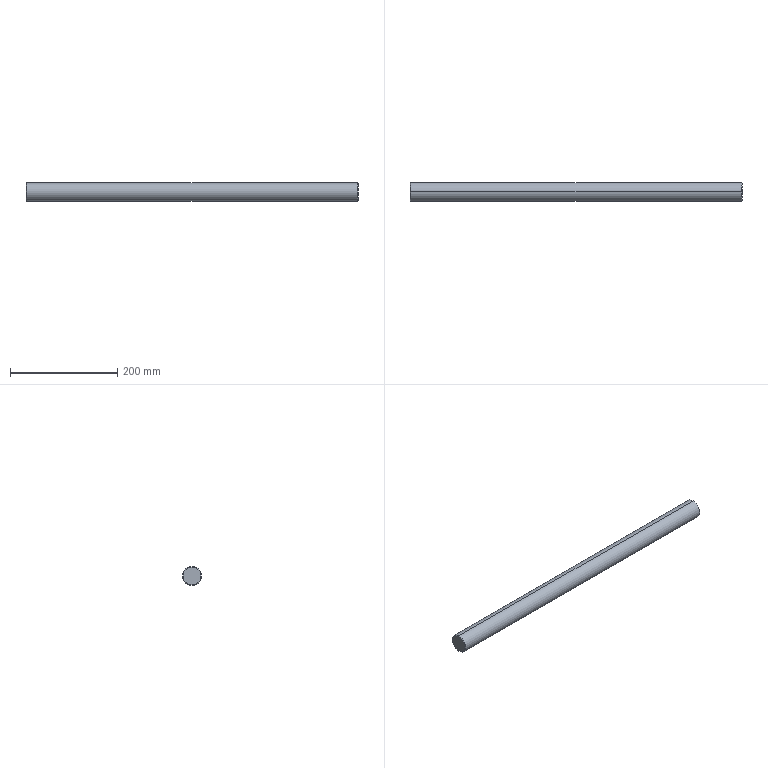Part | STEP file | PN_0034_driven shaft | 1 solid | 8 faces | box 620 x 35 x 35 mm | volume 596402 mm3 | cone 4 | cylinder 2 | plane 2 | commonest cylinder face diameters 35 x2
STEP:
#1=CARTESIAN_POINT('',(0.,0.,0.));
#2=DIRECTION('',(0.,0.,1.));
#3=DIRECTION('',(1.,0.,0.));
#4=AXIS2_PLACEMENT_3D('',#1,#2,#3);
#5=CARTESIAN_POINT('',(619.,0.,17.5));
#6=VERTEX_POINT('',#5);
#7=CARTESIAN_POINT('',(619.,0.,-17.5));
#8=VERTEX_POINT('',#7);
#9=CARTESIAN_POINT('',(619.,0.,0.));
#10=DIRECTION('',(-1.,0.,0.));
#11=DIRECTION('',(0.,0.,1.));
#12=AXIS2_PLACEMENT_3D('',#9,#10,#11);
#13=CIRCLE('',#12,17.5);
#14=CARTESIAN_POINT('',(620.,0.,0.));
#15=DIRECTION('',(-1.,0.,0.));
#16=DIRECTION('',(0.,0.,1.));
#17=AXIS2_PLACEMENT_3D('',#14,#15,#16);
#18=CYLINDRICAL_SURFACE('',#17,17.5);
#19=CARTESIAN_POINT('',(0.,1.));
#20=DIRECTION('',(1.,0.));
#21=VECTOR('',#20,1.);
#22=LINE('',#19,#21);
#23=(GEOMETRIC_REPRESENTATION_CONTEXT(2)PARAMETRIC_REPRESENTATION_CONTEXT()REPRESENTATION_CONTEXT('',''));
#24=DEFINITIONAL_REPRESENTATION('',(#22),#23);
#25=PCURVE('',#18,#24);
#26=CARTESIAN_POINT('',(619.,0.,0.));
#27=DIRECTION('',(-1.,0.,0.));
#28=DIRECTION('',(0.,0.,1.));
#29=AXIS2_PLACEMENT_3D('',#26,#27,#28);
#30=CONICAL_SURFACE('',#29,17.5,0.7854);
#31=CARTESIAN_POINT('',(0.,0.));
#32=DIRECTION('',(1.,0.));
#33=VECTOR('',#32,1.);
#34=LINE('',#31,#33);
#35=(GEOMETRIC_REPRESENTATION_CONTEXT(2)PARAMETRIC_REPRESENTATION_CONTEXT()REPRESENTATION_CONTEXT('',''));
#36=DEFINITIONAL_REPRESENTATION('',(#34),#35);
#37=PCURVE('',#30,#36);
#38=SURFACE_CURVE('',#13,(#25,#37),.PCURVE_S1.);
#39=EDGE_CURVE('',#6,#8,#38,.T.);
#40=ORIENTED_EDGE('',*,*,#39,.T.);
#41=CARTESIAN_POINT('',(1.,0.,-17.5));
#42=VERTEX_POINT('',#41);
#43=CARTESIAN_POINT('',(620.,0.,-17.5));
#44=DIRECTION('',(-1.,0.,0.));
#45=VECTOR('',#44,1.);
#46=LINE('',#43,#45);
#47=CARTESIAN_POINT('',(3.142,0.));
#48=DIRECTION('',(0.,1.));
#49=VECTOR('',#48,1.);
#50=LINE('',#47,#49);
#51=(GEOMETRIC_REPRESENTATION_CONTEXT(2)PARAMETRIC_REPRESENTATION_CONTEXT()REPRESENTATION_CONTEXT('',''));
#52=DEFINITIONAL_REPRESENTATION('',(#50),#51);
#53=PCURVE('',#18,#52);
#54=CARTESIAN_POINT('',(620.,0.,0.));
#55=DIRECTION('',(-1.,0.,0.));
#56=DIRECTION('',(0.,0.,1.));
#57=AXIS2_PLACEMENT_3D('',#54,#55,#56);
#58=CYLINDRICAL_SURFACE('',#57,17.5);
#59=CARTESIAN_POINT('',(3.142,0.));
#60=DIRECTION('',(0.,1.));
#61=VECTOR('',#60,1.);
#62=LINE('',#59,#61);
#63=(GEOMETRIC_REPRESENTATION_CONTEXT(2)PARAMETRIC_REPRESENTATION_CONTEXT()REPRESENTATION_CONTEXT('',''));
#64=DEFINITIONAL_REPRESENTATION('',(#62),#63);
#65=PCURVE('',#58,#64);
#66=SURFACE_CURVE('',#46,(#53,#65),.PCURVE_S1.);
#67=EDGE_CURVE('',#8,#42,#66,.T.);
#68=ORIENTED_EDGE('',*,*,#67,.T.);
#69=CARTESIAN_POINT('',(1.,0.,17.5));
#70=VERTEX_POINT('',#69);
#71=CARTESIAN_POINT('',(1.,0.,0.));
#72=DIRECTION('',(1.,0.,0.));
#73=DIRECTION('',(0.,0.,1.));
#74=AXIS2_PLACEMENT_3D('',#71,#72,#73);
#75=CIRCLE('',#74,17.5);
#76=CARTESIAN_POINT('',(6.283,619.));
#77=DIRECTION('',(-1.,0.));
#78=VECTOR('',#77,1.);
#79=LINE('',#76,#78);
#80=(GEOMETRIC_REPRESENTATION_CONTEXT(2)PARAMETRIC_REPRESENTATION_CONTEXT()REPRESENTATION_CONTEXT('',''));
#81=DEFINITIONAL_REPRESENTATION('',(#79),#80);
#82=PCURVE('',#18,#81);
#83=CARTESIAN_POINT('',(1.,0.,0.));
#84=DIRECTION('',(1.,0.,0.));
#85=DIRECTION('',(0.,0.,-1.));
#86=AXIS2_PLACEMENT_3D('',#83,#84,#85);
#87=CONICAL_SURFACE('',#86,17.5,0.7854);
#88=CARTESIAN_POINT('',(-3.142,0.));
#89=DIRECTION('',(1.,0.));
#90=VECTOR('',#89,1.);
#91=LINE('',#88,#90);
#92=(GEOMETRIC_REPRESENTATION_CONTEXT(2)PARAMETRIC_REPRESENTATION_CONTEXT()REPRESENTATION_CONTEXT('',''));
#93=DEFINITIONAL_REPRESENTATION('',(#91),#92);
#94=PCURVE('',#87,#93);
#95=SURFACE_CURVE('',#75,(#82,#94),.PCURVE_S1.);
#96=EDGE_CURVE('',#42,#70,#95,.T.);
#97=ORIENTED_EDGE('',*,*,#96,.T.);
#98=CARTESIAN_POINT('',(620.,0.,17.5));
#99=DIRECTION('',(-1.,0.,0.));
#100=VECTOR('',#99,1.);
#101=LINE('',#98,#100);
#102=CARTESIAN_POINT('',(0.,0.));
#103=DIRECTION('',(0.,1.));
#104=VECTOR('',#103,1.);
#105=LINE('',#102,#104);
#106=(GEOMETRIC_REPRESENTATION_CONTEXT(2)PARAMETRIC_REPRESENTATION_CONTEXT()REPRESENTATION_CONTEXT('',''));
#107=DEFINITIONAL_REPRESENTATION('',(#105),#106);
#108=PCURVE('',#18,#107);
#109=CARTESIAN_POINT('',(6.283,0.));
#110=DIRECTION('',(0.,1.));
#111=VECTOR('',#110,1.);
#112=LINE('',#109,#111);
#113=(GEOMETRIC_REPRESENTATION_CONTEXT(2)PARAMETRIC_REPRESENTATION_CONTEXT()REPRESENTATION_CONTEXT('',''));
#114=DEFINITIONAL_REPRESENTATION('',(#112),#113);
#115=PCURVE('',#58,#114);
#116=SURFACE_CURVE('',#101,(#108,#115),.PCURVE_S1.);
#117=EDGE_CURVE('',#6,#70,#116,.T.);
#118=ORIENTED_EDGE('',*,*,#117,.F.);
#119=EDGE_LOOP('',(#40,#68,#97,#118));
#120=FACE_BOUND('',#119,.T.);
#121=ADVANCED_FACE('',(#120),#18,.T.);
#122=CARTESIAN_POINT('',(0.,0.,-16.5));
#123=VERTEX_POINT('',#122);
#124=CARTESIAN_POINT('',(0.,0.,16.5));
#125=VERTEX_POINT('',#124);
#126=CARTESIAN_POINT('',(0.,0.,0.));
#127=DIRECTION('',(1.,0.,0.));
#128=DIRECTION('',(0.,0.,-1.));
#129=AXIS2_PLACEMENT_3D('',#126,#127,#128);
#130=CIRCLE('',#129,16.5);
#131=CARTESIAN_POINT('',(0.,-1.));
#132=DIRECTION('',(1.,0.));
#133=VECTOR('',#132,1.);
#134=LINE('',#131,#133);
#135=(GEOMETRIC_REPRESENTATION_CONTEXT(2)PARAMETRIC_REPRESENTATION_CONTEXT()REPRESENTATION_CONTEXT('',''));
#136=DEFINITIONAL_REPRESENTATION('',(#134),#135);
#137=PCURVE('',#87,#136);
#138=CARTESIAN_POINT('',(0.,0.,0.));
#139=DIRECTION('',(1.,0.,0.));
#140=DIRECTION('',(0.,0.,-1.));
#141=AXIS2_PLACEMENT_3D('',#138,#139,#140);
#142=PLANE('',#141);
#143=CARTESIAN_POINT('',(0.,0.));
#144=DIRECTION('',(1.,0.));
#145=AXIS2_PLACEMENT_2D('',#143,#144);
#146=CIRCLE('',#145,16.5);
#147=(GEOMETRIC_REPRESENTATION_CONTEXT(2)PARAMETRIC_REPRESENTATION_CONTEXT()REPRESENTATION_CONTEXT('',''));
#148=DEFINITIONAL_REPRESENTATION('',(#146),#147);
#149=PCURVE('',#142,#148);
#150=SURFACE_CURVE('',#130,(#137,#149),.PCURVE_S1.);
#151=EDGE_CURVE('',#123,#125,#150,.T.);
#152=ORIENTED_EDGE('',*,*,#151,.T.);
#153=CARTESIAN_POINT('',(1.,0.,17.5));
#154=DIRECTION('',(0.7071,0.,0.7071));
#155=VECTOR('',#154,1.);
#156=LINE('',#153,#155);
#157=CARTESIAN_POINT('',(3.142,0.));
#158=DIRECTION('',(0.,1.));
#159=VECTOR('',#158,1.);
#160=LINE('',#157,#159);
#161=(GEOMETRIC_REPRESENTATION_CONTEXT(2)PARAMETRIC_REPRESENTATION_CONTEXT()REPRESENTATION_CONTEXT('',''));
#162=DEFINITIONAL_REPRESENTATION('',(#160),#161);
#163=PCURVE('',#87,#162);
#164=CARTESIAN_POINT('',(1.,0.,0.));
#165=DIRECTION('',(1.,0.,0.));
#166=DIRECTION('',(0.,0.,-1.));
#167=AXIS2_PLACEMENT_3D('',#164,#165,#166);
#168=CONICAL_SURFACE('',#167,17.5,0.7854);
#169=CARTESIAN_POINT('',(3.142,0.));
#170=DIRECTION('',(0.,1.));
#171=VECTOR('',#170,1.);
#172=LINE('',#169,#171);
#173=(GEOMETRIC_REPRESENTATION_CONTEXT(2)PARAMETRIC_REPRESENTATION_CONTEXT()REPRESENTATION_CONTEXT('',''));
#174=DEFINITIONAL_REPRESENTATION('',(#172),#173);
#175=PCURVE('',#168,#174);
#176=SURFACE_CURVE('',#156,(#163,#175),.PCURVE_S1.);
#177=EDGE_CURVE('',#125,#70,#176,.T.);
#178=ORIENTED_EDGE('',*,*,#177,.T.);
#179=ORIENTED_EDGE('',*,*,#96,.F.);
#180=CARTESIAN_POINT('',(1.,0.,-17.5));
#181=DIRECTION('',(0.7071,0.,-0.7071));
#182=VECTOR('',#181,1.);
#183=LINE('',#180,#182);
#184=CARTESIAN_POINT('',(0.,0.));
#185=DIRECTION('',(0.,1.));
#186=VECTOR('',#185,1.);
#187=LINE('',#184,#186);
#188=(GEOMETRIC_REPRESENTATION_CONTEXT(2)PARAMETRIC_REPRESENTATION_CONTEXT()REPRESENTATION_CONTEXT('',''));
#189=DEFINITIONAL_REPRESENTATION('',(#187),#188);
#190=PCURVE('',#87,#189);
#191=CARTESIAN_POINT('',(6.283,0.));
#192=DIRECTION('',(0.,1.));
#193=VECTOR('',#192,1.);
#194=LINE('',#191,#193);
#195=(GEOMETRIC_REPRESENTATION_CONTEXT(2)PARAMETRIC_REPRESENTATION_CONTEXT()REPRESENTATION_CONTEXT('',''));
#196=DEFINITIONAL_REPRESENTATION('',(#194),#195);
#197=PCURVE('',#168,#196);
#198=SURFACE_CURVE('',#183,(#190,#197),.PCURVE_S1.);
#199=EDGE_CURVE('',#123,#42,#198,.T.);
#200=ORIENTED_EDGE('',*,*,#199,.F.);
#201=EDGE_LOOP('',(#152,#178,#179,#200));
#202=FACE_BOUND('',#201,.T.);
#203=ADVANCED_FACE('',(#202),#87,.T.);
#204=CARTESIAN_POINT('',(620.,0.,16.5));
#205=VERTEX_POINT('',#204);
#206=CARTESIAN_POINT('',(620.,0.,-16.5));
#207=VERTEX_POINT('',#206);
#208=CARTESIAN_POINT('',(620.,0.,0.));
#209=DIRECTION('',(-1.,0.,0.));
#210=DIRECTION('',(0.,0.,1.));
#211=AXIS2_PLACEMENT_3D('',#208,#209,#210);
#212=CIRCLE('',#211,16.5);
#213=CARTESIAN_POINT('',(0.,-1.));
#214=DIRECTION('',(1.,0.));
#215=VECTOR('',#214,1.);
#216=LINE('',#213,#215);
#217=(GEOMETRIC_REPRESENTATION_CONTEXT(2)PARAMETRIC_REPRESENTATION_CONTEXT()REPRESENTATION_CONTEXT('',''));
#218=DEFINITIONAL_REPRESENTATION('',(#216),#217);
#219=PCURVE('',#30,#218);
#220=CARTESIAN_POINT('',(620.,0.,0.));
#221=DIRECTION('',(1.,0.,0.));
#222=DIRECTION('',(0.,0.,-1.));
#223=AXIS2_PLACEMENT_3D('',#220,#221,#222);
#224=PLANE('',#223);
#225=CARTESIAN_POINT('',(-16.5,0.));
#226=CARTESIAN_POINT('',(-16.5,28.579));
#227=CARTESIAN_POINT('',(8.25,14.289));
#228=CARTESIAN_POINT('',(33.,0.));
#229=CARTESIAN_POINT('',(8.25,-14.289));
#230=CARTESIAN_POINT('',(-16.5,-28.579));
#231=CARTESIAN_POINT('',(-16.5,0.));
#232=(BOUNDED_CURVE()B_SPLINE_CURVE(2,(#225,#226,#227,#228,#229,#230,#231),.UNSPECIFIED.,.T.,.F.)B_SPLINE_CURVE_WITH_KNOTS((1,2,2,2,2,1),(-2.094,0.,2.094,4.189,6.283,8.378),.UNSPECIFIED.)CURVE()GEOMETRIC_REPRESENTATION_ITEM()RATIONAL_B_SPLINE_CURVE((1.,0.5,1.,0.5,1.,0.5,1.))REPRESENTATION_ITEM(''));
#233=(GEOMETRIC_REPRESENTATION_CONTEXT(2)PARAMETRIC_REPRESENTATION_CONTEXT()REPRESENTATION_CONTEXT('',''));
#234=DEFINITIONAL_REPRESENTATION('',(#232),#233);
#235=PCURVE('',#224,#234);
#236=SURFACE_CURVE('',#212,(#219,#235),.PCURVE_S1.);
#237=EDGE_CURVE('',#205,#207,#236,.T.);
#238=ORIENTED_EDGE('',*,*,#237,.T.);
#239=CARTESIAN_POINT('',(619.,0.,-17.5));
#240=DIRECTION('',(-0.7071,0.,-0.7071));
#241=VECTOR('',#240,1.);
#242=LINE('',#239,#241);
#243=CARTESIAN_POINT('',(3.142,0.));
#244=DIRECTION('',(0.,1.));
#245=VECTOR('',#244,1.);
#246=LINE('',#243,#245);
#247=(GEOMETRIC_REPRESENTATION_CONTEXT(2)PARAMETRIC_REPRESENTATION_CONTEXT()REPRESENTATION_CONTEXT('',''));
#248=DEFINITIONAL_REPRESENTATION('',(#246),#247);
#249=PCURVE('',#30,#248);
#250=CARTESIAN_POINT('',(619.,0.,0.));
#251=DIRECTION('',(-1.,0.,0.));
#252=DIRECTION('',(0.,0.,1.));
#253=AXIS2_PLACEMENT_3D('',#250,#251,#252);
#254=CONICAL_SURFACE('',#253,17.5,0.7854);
#255=CARTESIAN_POINT('',(3.142,0.));
#256=DIRECTION('',(0.,1.));
#257=VECTOR('',#256,1.);
#258=LINE('',#255,#257);
#259=(GEOMETRIC_REPRESENTATION_CONTEXT(2)PARAMETRIC_REPRESENTATION_CONTEXT()REPRESENTATION_CONTEXT('',''));
#260=DEFINITIONAL_REPRESENTATION('',(#258),#259);
#261=PCURVE('',#254,#260);
#262=SURFACE_CURVE('',#242,(#249,#261),.PCURVE_S1.);
#263=EDGE_CURVE('',#207,#8,#262,.T.);
#264=ORIENTED_EDGE('',*,*,#263,.T.);
#265=ORIENTED_EDGE('',*,*,#39,.F.);
#266=CARTESIAN_POINT('',(619.,0.,17.5));
#267=DIRECTION('',(-0.7071,0.,0.7071));
#268=VECTOR('',#267,1.);
#269=LINE('',#266,#268);
#270=CARTESIAN_POINT('',(0.,0.));
#271=DIRECTION('',(0.,1.));
#272=VECTOR('',#271,1.);
#273=LINE('',#270,#272);
#274=(GEOMETRIC_REPRESENTATION_CONTEXT(2)PARAMETRIC_REPRESENTATION_CONTEXT()REPRESENTATION_CONTEXT('',''));
#275=DEFINITIONAL_REPRESENTATION('',(#273),#274);
#276=PCURVE('',#30,#275);
#277=CARTESIAN_POINT('',(6.283,0.));
#278=DIRECTION('',(0.,1.));
#279=VECTOR('',#278,1.);
#280=LINE('',#277,#279);
#281=(GEOMETRIC_REPRESENTATION_CONTEXT(2)PARAMETRIC_REPRESENTATION_CONTEXT()REPRESENTATION_CONTEXT('',''));
#282=DEFINITIONAL_REPRESENTATION('',(#280),#281);
#283=PCURVE('',#254,#282);
#284=SURFACE_CURVE('',#269,(#276,#283),.PCURVE_S1.);
#285=EDGE_CURVE('',#205,#6,#284,.T.);
#286=ORIENTED_EDGE('',*,*,#285,.F.);
#287=EDGE_LOOP('',(#238,#264,#265,#286));
#288=FACE_BOUND('',#287,.T.);
#289=ADVANCED_FACE('',(#288),#30,.T.);
#290=ORIENTED_EDGE('',*,*,#67,.F.);
#291=CARTESIAN_POINT('',(619.,0.,0.));
#292=DIRECTION('',(-1.,0.,0.));
#293=DIRECTION('',(0.,0.,1.));
#294=AXIS2_PLACEMENT_3D('',#291,#292,#293);
#295=CIRCLE('',#294,17.5);
#296=CARTESIAN_POINT('',(0.,1.));
#297=DIRECTION('',(1.,0.));
#298=VECTOR('',#297,1.);
#299=LINE('',#296,#298);
#300=(GEOMETRIC_REPRESENTATION_CONTEXT(2)PARAMETRIC_REPRESENTATION_CONTEXT()REPRESENTATION_CONTEXT('',''));
#301=DEFINITIONAL_REPRESENTATION('',(#299),#300);
#302=PCURVE('',#58,#301);
#303=CARTESIAN_POINT('',(0.,0.));
#304=DIRECTION('',(1.,0.));
#305=VECTOR('',#304,1.);
#306=LINE('',#303,#305);
#307=(GEOMETRIC_REPRESENTATION_CONTEXT(2)PARAMETRIC_REPRESENTATION_CONTEXT()REPRESENTATION_CONTEXT('',''));
#308=DEFINITIONAL_REPRESENTATION('',(#306),#307);
#309=PCURVE('',#254,#308);
#310=SURFACE_CURVE('',#295,(#302,#309),.PCURVE_S1.);
#311=EDGE_CURVE('',#8,#6,#310,.T.);
#312=ORIENTED_EDGE('',*,*,#311,.T.);
#313=ORIENTED_EDGE('',*,*,#117,.T.);
#314=CARTESIAN_POINT('',(1.,0.,0.));
#315=DIRECTION('',(1.,0.,0.));
#316=DIRECTION('',(0.,0.,1.));
#317=AXIS2_PLACEMENT_3D('',#314,#315,#316);
#318=CIRCLE('',#317,17.5);
#319=CARTESIAN_POINT('',(6.283,619.));
#320=DIRECTION('',(-1.,0.));
#321=VECTOR('',#320,1.);
#322=LINE('',#319,#321);
#323=(GEOMETRIC_REPRESENTATION_CONTEXT(2)PARAMETRIC_REPRESENTATION_CONTEXT()REPRESENTATION_CONTEXT('',''));
#324=DEFINITIONAL_REPRESENTATION('',(#322),#323);
#325=PCURVE('',#58,#324);
#326=CARTESIAN_POINT('',(3.142,0.));
#327=DIRECTION('',(1.,0.));
#328=VECTOR('',#327,1.);
#329=LINE('',#326,#328);
#330=(GEOMETRIC_REPRESENTATION_CONTEXT(2)PARAMETRIC_REPRESENTATION_CONTEXT()REPRESENTATION_CONTEXT('',''));
#331=DEFINITIONAL_REPRESENTATION('',(#329),#330);
#332=PCURVE('',#168,#331);
#333=SURFACE_CURVE('',#318,(#325,#332),.PCURVE_S1.);
#334=EDGE_CURVE('',#70,#42,#333,.T.);
#335=ORIENTED_EDGE('',*,*,#334,.T.);
#336=EDGE_LOOP('',(#290,#312,#313,#335));
#337=FACE_BOUND('',#336,.T.);
#338=ADVANCED_FACE('',(#337),#58,.T.);
#339=ORIENTED_EDGE('',*,*,#177,.F.);
#340=CARTESIAN_POINT('',(0.,0.,0.));
#341=DIRECTION('',(1.,0.,0.));
#342=DIRECTION('',(0.,0.,-1.));
#343=AXIS2_PLACEMENT_3D('',#340,#341,#342);
#344=CIRCLE('',#343,16.5);
#345=CARTESIAN_POINT('',(0.,-1.));
#346=DIRECTION('',(1.,0.));
#347=VECTOR('',#346,1.);
#348=LINE('',#345,#347);
#349=(GEOMETRIC_REPRESENTATION_CONTEXT(2)PARAMETRIC_REPRESENTATION_CONTEXT()REPRESENTATION_CONTEXT('',''));
#350=DEFINITIONAL_REPRESENTATION('',(#348),#349);
#351=PCURVE('',#168,#350);
#352=CARTESIAN_POINT('',(0.,0.));
#353=DIRECTION('',(1.,0.));
#354=AXIS2_PLACEMENT_2D('',#352,#353);
#355=CIRCLE('',#354,16.5);
#356=(GEOMETRIC_REPRESENTATION_CONTEXT(2)PARAMETRIC_REPRESENTATION_CONTEXT()REPRESENTATION_CONTEXT('',''));
#357=DEFINITIONAL_REPRESENTATION('',(#355),#356);
#358=PCURVE('',#142,#357);
#359=SURFACE_CURVE('',#344,(#351,#358),.PCURVE_S1.);
#360=EDGE_CURVE('',#125,#123,#359,.T.);
#361=ORIENTED_EDGE('',*,*,#360,.T.);
#362=ORIENTED_EDGE('',*,*,#199,.T.);
#363=ORIENTED_EDGE('',*,*,#334,.F.);
#364=EDGE_LOOP('',(#339,#361,#362,#363));
#365=FACE_BOUND('',#364,.T.);
#366=ADVANCED_FACE('',(#365),#168,.T.);
#367=ORIENTED_EDGE('',*,*,#263,.F.);
#368=CARTESIAN_POINT('',(620.,0.,0.));
#369=DIRECTION('',(-1.,0.,0.));
#370=DIRECTION('',(0.,0.,1.));
#371=AXIS2_PLACEMENT_3D('',#368,#369,#370);
#372=CIRCLE('',#371,16.5);
#373=CARTESIAN_POINT('',(0.,-1.));
#374=DIRECTION('',(1.,0.));
#375=VECTOR('',#374,1.);
#376=LINE('',#373,#375);
#377=(GEOMETRIC_REPRESENTATION_CONTEXT(2)PARAMETRIC_REPRESENTATION_CONTEXT()REPRESENTATION_CONTEXT('',''));
#378=DEFINITIONAL_REPRESENTATION('',(#376),#377);
#379=PCURVE('',#254,#378);
#380=CARTESIAN_POINT('',(-16.5,0.));
#381=CARTESIAN_POINT('',(-16.5,28.579));
#382=CARTESIAN_POINT('',(8.25,14.289));
#383=CARTESIAN_POINT('',(33.,0.));
#384=CARTESIAN_POINT('',(8.25,-14.289));
#385=CARTESIAN_POINT('',(-16.5,-28.579));
#386=CARTESIAN_POINT('',(-16.5,0.));
#387=(BOUNDED_CURVE()B_SPLINE_CURVE(2,(#380,#381,#382,#383,#384,#385,#386),.UNSPECIFIED.,.T.,.F.)B_SPLINE_CURVE_WITH_KNOTS((1,2,2,2,2,1),(-2.094,0.,2.094,4.189,6.283,8.378),.UNSPECIFIED.)CURVE()GEOMETRIC_REPRESENTATION_ITEM()RATIONAL_B_SPLINE_CURVE((1.,0.5,1.,0.5,1.,0.5,1.))REPRESENTATION_ITEM(''));
#388=(GEOMETRIC_REPRESENTATION_CONTEXT(2)PARAMETRIC_REPRESENTATION_CONTEXT()REPRESENTATION_CONTEXT('',''));
#389=DEFINITIONAL_REPRESENTATION('',(#387),#388);
#390=PCURVE('',#224,#389);
#391=SURFACE_CURVE('',#372,(#379,#390),.PCURVE_S1.);
#392=EDGE_CURVE('',#207,#205,#391,.T.);
#393=ORIENTED_EDGE('',*,*,#392,.T.);
#394=ORIENTED_EDGE('',*,*,#285,.T.);
#395=ORIENTED_EDGE('',*,*,#311,.F.);
#396=EDGE_LOOP('',(#367,#393,#394,#395));
#397=FACE_BOUND('',#396,.T.);
#398=ADVANCED_FACE('',(#397),#254,.T.);
#399=ORIENTED_EDGE('',*,*,#151,.F.);
#400=ORIENTED_EDGE('',*,*,#360,.F.);
#401=EDGE_LOOP('',(#399,#400));
#402=FACE_BOUND('',#401,.T.);
#403=ADVANCED_FACE('',(#402),#142,.F.);
#404=ORIENTED_EDGE('',*,*,#237,.F.);
#405=ORIENTED_EDGE('',*,*,#392,.F.);
#406=EDGE_LOOP('',(#404,#405));
#407=FACE_BOUND('',#406,.T.);
#408=ADVANCED_FACE('',(#407),#224,.T.);
#409=CLOSED_SHELL('',(#121,#203,#289,#338,#366,#398,#403,#408));
#410=MANIFOLD_SOLID_BREP('',#409);
#411=(LENGTH_UNIT()NAMED_UNIT(*)SI_UNIT(.MILLI.,.METRE.));
#412=UNCERTAINTY_MEASURE_WITH_UNIT(LENGTH_MEASURE(0.0000001),#411,'','');
#413=(NAMED_UNIT(*)PLANE_ANGLE_UNIT()SI_UNIT($,.RADIAN.));
#414=(NAMED_UNIT(*)SI_UNIT($,.STERADIAN.)SOLID_ANGLE_UNIT());
#415=(GEOMETRIC_REPRESENTATION_CONTEXT(3)GLOBAL_UNCERTAINTY_ASSIGNED_CONTEXT((#412))GLOBAL_UNIT_ASSIGNED_CONTEXT((#411,#413,#414))REPRESENTATION_CONTEXT('',''));
#416=ADVANCED_BREP_SHAPE_REPRESENTATION('',(#4,#410),#415);